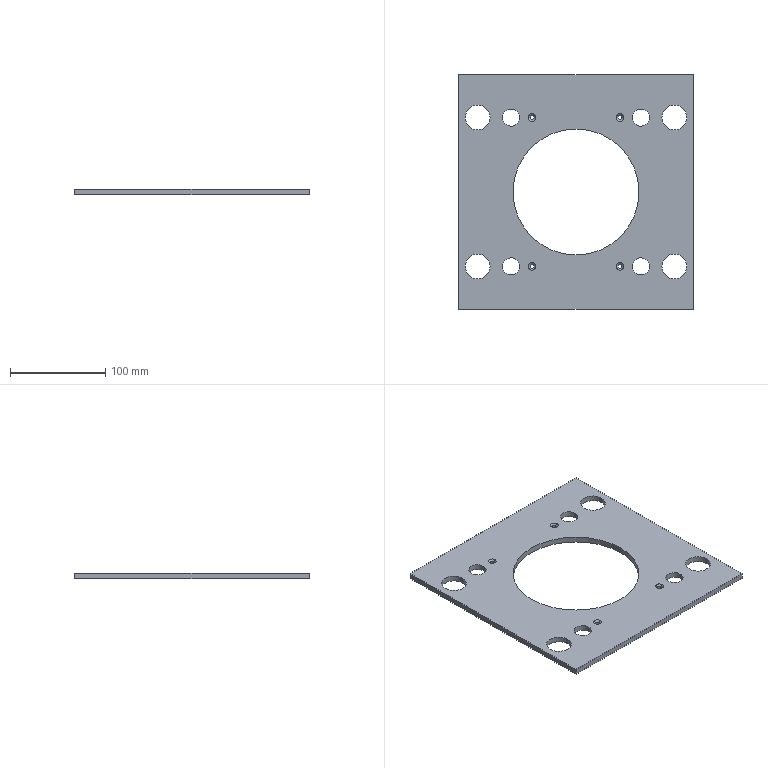Part | STEP file | Insulating plate | 1 solid | 40 faces | box 246 x 246 x 6 mm | volume 261647 mm3 | cylinder 26 | cone 8 | plane 6 | commonest cylinder face diameters 4.5 x8 18 x8 26 x8 132 x2